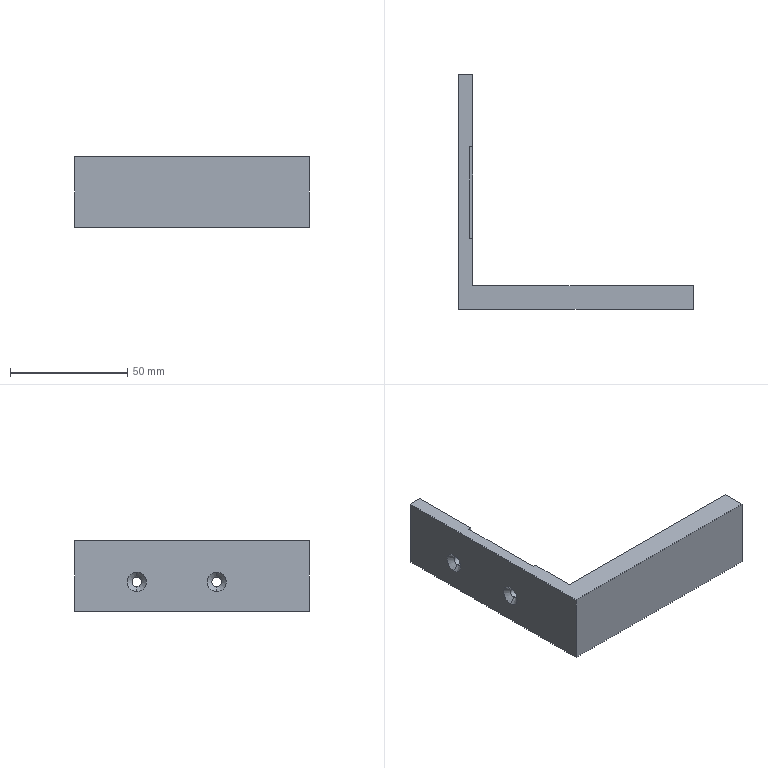Part | SolidWorks | features ICE 2, Chamfer 1, Extrusion 1 | 1 solid | 20 faces | box 100 x 100 x 30 mm | volume 45451 mm3 | plane 12 | cone 4 | cylinder 4 | commonest cylinder face diameters 4 x4
STEP:
#1=CARTESIAN_POINT('',(2.1,73.5,10.5));
#2=VERTEX_POINT('',#1);
#3=CARTESIAN_POINT('',(2.1,73.5,14.5));
#4=VERTEX_POINT('',#3);
#5=CARTESIAN_POINT('',(2.1,73.5,12.5));
#6=DIRECTION('',(-1.,0.,0.));
#7=DIRECTION('',(0.,0.,-1.));
#8=AXIS2_PLACEMENT_3D('',#5,#6,#7);
#9=CIRCLE('',#8,2.);
#10=EDGE_CURVE('',#2,#4,#9,.T.);
#11=ORIENTED_EDGE('',*,*,#10,.F.);
#12=CARTESIAN_POINT('',(0.,73.5,8.4));
#13=VERTEX_POINT('',#12);
#14=CARTESIAN_POINT('',(2.1,73.5,10.5));
#15=DIRECTION('',(-0.7071,0.,-0.7071));
#16=VECTOR('',#15,1000.);
#17=LINE('',#14,#16);
#18=EDGE_CURVE('',#2,#13,#17,.T.);
#19=ORIENTED_EDGE('',*,*,#18,.T.);
#20=CARTESIAN_POINT('',(0.,73.5,16.6));
#21=VERTEX_POINT('',#20);
#22=CARTESIAN_POINT('',(0.,73.5,12.5));
#23=DIRECTION('',(1.,0.,0.));
#24=DIRECTION('',(0.,0.,-1.));
#25=AXIS2_PLACEMENT_3D('',#22,#23,#24);
#26=CIRCLE('',#25,4.1);
#27=EDGE_CURVE('',#21,#13,#26,.T.);
#28=ORIENTED_EDGE('',*,*,#27,.F.);
#29=CARTESIAN_POINT('',(2.1,73.5,14.5));
#30=DIRECTION('',(-0.7071,0.,0.7071));
#31=VECTOR('',#30,1000.);
#32=LINE('',#29,#31);
#33=EDGE_CURVE('',#4,#21,#32,.T.);
#34=ORIENTED_EDGE('',*,*,#33,.F.);
#35=EDGE_LOOP('',(#11,#19,#28,#34));
#36=FACE_OUTER_BOUND('',#35,.T.);
#37=CARTESIAN_POINT('',(2.1,73.5,12.5));
#38=DIRECTION('',(-1.,0.,0.));
#39=DIRECTION('',(0.,0.,1.));
#40=AXIS2_PLACEMENT_3D('',#37,#38,#39);
#41=CONICAL_SURFACE('',#40,2.,0.7854);
#42=ADVANCED_FACE('',(#36),#41,.F.);
#43=CARTESIAN_POINT('',(2.1,39.5,10.5));
#44=VERTEX_POINT('',#43);
#45=CARTESIAN_POINT('',(2.1,39.5,14.5));
#46=VERTEX_POINT('',#45);
#47=CARTESIAN_POINT('',(2.1,39.5,12.5));
#48=DIRECTION('',(-1.,0.,0.));
#49=DIRECTION('',(0.,0.,-1.));
#50=AXIS2_PLACEMENT_3D('',#47,#48,#49);
#51=CIRCLE('',#50,2.);
#52=EDGE_CURVE('',#44,#46,#51,.T.);
#53=ORIENTED_EDGE('',*,*,#52,.F.);
#54=CARTESIAN_POINT('',(0.,39.5,8.4));
#55=VERTEX_POINT('',#54);
#56=CARTESIAN_POINT('',(2.1,39.5,10.5));
#57=DIRECTION('',(-0.7071,0.,-0.7071));
#58=VECTOR('',#57,1000.);
#59=LINE('',#56,#58);
#60=EDGE_CURVE('',#44,#55,#59,.T.);
#61=ORIENTED_EDGE('',*,*,#60,.T.);
#62=CARTESIAN_POINT('',(0.,39.5,16.6));
#63=VERTEX_POINT('',#62);
#64=CARTESIAN_POINT('',(0.,39.5,12.5));
#65=DIRECTION('',(1.,0.,0.));
#66=DIRECTION('',(0.,0.,-1.));
#67=AXIS2_PLACEMENT_3D('',#64,#65,#66);
#68=CIRCLE('',#67,4.1);
#69=EDGE_CURVE('',#63,#55,#68,.T.);
#70=ORIENTED_EDGE('',*,*,#69,.F.);
#71=CARTESIAN_POINT('',(2.1,39.5,14.5));
#72=DIRECTION('',(-0.7071,0.,0.7071));
#73=VECTOR('',#72,1000.);
#74=LINE('',#71,#73);
#75=EDGE_CURVE('',#46,#63,#74,.T.);
#76=ORIENTED_EDGE('',*,*,#75,.F.);
#77=EDGE_LOOP('',(#53,#61,#70,#76));
#78=FACE_OUTER_BOUND('',#77,.T.);
#79=CARTESIAN_POINT('',(2.1,39.5,12.5));
#80=DIRECTION('',(-1.,0.,0.));
#81=DIRECTION('',(0.,0.,1.));
#82=AXIS2_PLACEMENT_3D('',#79,#80,#81);
#83=CONICAL_SURFACE('',#82,2.,0.7854);
#84=ADVANCED_FACE('',(#78),#83,.F.);
#85=CARTESIAN_POINT('',(6.,39.5,10.5));
#86=VERTEX_POINT('',#85);
#87=CARTESIAN_POINT('',(6.,39.5,14.5));
#88=VERTEX_POINT('',#87);
#89=CARTESIAN_POINT('',(6.,39.5,12.5));
#90=DIRECTION('',(-1.,0.,0.));
#91=DIRECTION('',(0.,-1.,0.));
#92=AXIS2_PLACEMENT_3D('',#89,#90,#91);
#93=CIRCLE('',#92,2.);
#94=EDGE_CURVE('',#86,#88,#93,.T.);
#95=ORIENTED_EDGE('',*,*,#94,.F.);
#96=CARTESIAN_POINT('',(100.,39.5,10.5));
#97=DIRECTION('',(-1.,0.,0.));
#98=VECTOR('',#97,1000.);
#99=LINE('',#96,#98);
#100=EDGE_CURVE('',#86,#44,#99,.T.);
#101=ORIENTED_EDGE('',*,*,#100,.T.);
#102=ORIENTED_EDGE('',*,*,#52,.T.);
#103=CARTESIAN_POINT('',(100.,39.5,14.5));
#104=DIRECTION('',(-1.,0.,0.));
#105=VECTOR('',#104,1000.);
#106=LINE('',#103,#105);
#107=EDGE_CURVE('',#88,#46,#106,.T.);
#108=ORIENTED_EDGE('',*,*,#107,.F.);
#109=EDGE_LOOP('',(#95,#101,#102,#108));
#110=FACE_OUTER_BOUND('',#109,.T.);
#111=CARTESIAN_POINT('',(100.,39.5,12.5));
#112=DIRECTION('',(-1.,0.,0.));
#113=DIRECTION('',(0.,0.,1.));
#114=AXIS2_PLACEMENT_3D('',#111,#112,#113);
#115=CYLINDRICAL_SURFACE('',#114,2.);
#116=ADVANCED_FACE('',(#110),#115,.F.);
#117=CARTESIAN_POINT('',(6.,73.5,10.5));
#118=VERTEX_POINT('',#117);
#119=CARTESIAN_POINT('',(6.,73.5,14.5));
#120=VERTEX_POINT('',#119);
#121=CARTESIAN_POINT('',(6.,73.5,12.5));
#122=DIRECTION('',(-1.,0.,0.));
#123=DIRECTION('',(0.,-1.,0.));
#124=AXIS2_PLACEMENT_3D('',#121,#122,#123);
#125=CIRCLE('',#124,2.);
#126=EDGE_CURVE('',#118,#120,#125,.T.);
#127=ORIENTED_EDGE('',*,*,#126,.F.);
#128=CARTESIAN_POINT('',(100.,73.5,10.5));
#129=DIRECTION('',(-1.,0.,0.));
#130=VECTOR('',#129,1000.);
#131=LINE('',#128,#130);
#132=EDGE_CURVE('',#118,#2,#131,.T.);
#133=ORIENTED_EDGE('',*,*,#132,.T.);
#134=ORIENTED_EDGE('',*,*,#10,.T.);
#135=CARTESIAN_POINT('',(100.,73.5,14.5));
#136=DIRECTION('',(-1.,0.,0.));
#137=VECTOR('',#136,1000.);
#138=LINE('',#135,#137);
#139=EDGE_CURVE('',#120,#4,#138,.T.);
#140=ORIENTED_EDGE('',*,*,#139,.F.);
#141=EDGE_LOOP('',(#127,#133,#134,#140));
#142=FACE_OUTER_BOUND('',#141,.T.);
#143=CARTESIAN_POINT('',(100.,73.5,12.5));
#144=DIRECTION('',(-1.,0.,0.));
#145=DIRECTION('',(0.,0.,1.));
#146=AXIS2_PLACEMENT_3D('',#143,#144,#145);
#147=CYLINDRICAL_SURFACE('',#146,2.);
#148=ADVANCED_FACE('',(#142),#147,.F.);
#149=ORIENTED_EDGE('',*,*,#69,.T.);
#150=CARTESIAN_POINT('',(0.,39.5,12.5));
#151=DIRECTION('',(1.,0.,0.));
#152=DIRECTION('',(0.,0.,-1.));
#153=AXIS2_PLACEMENT_3D('',#150,#151,#152);
#154=CIRCLE('',#153,4.1);
#155=EDGE_CURVE('',#55,#63,#154,.T.);
#156=ORIENTED_EDGE('',*,*,#155,.T.);
#157=EDGE_LOOP('',(#149,#156));
#158=FACE_BOUND('',#157,.T.);
#159=ORIENTED_EDGE('',*,*,#27,.T.);
#160=CARTESIAN_POINT('',(0.,73.5,12.5));
#161=DIRECTION('',(1.,0.,0.));
#162=DIRECTION('',(0.,0.,-1.));
#163=AXIS2_PLACEMENT_3D('',#160,#161,#162);
#164=CIRCLE('',#163,4.1);
#165=EDGE_CURVE('',#13,#21,#164,.T.);
#166=ORIENTED_EDGE('',*,*,#165,.T.);
#167=EDGE_LOOP('',(#159,#166));
#168=FACE_BOUND('',#167,.T.);
#169=CARTESIAN_POINT('',(0.,100.,0.));
#170=VERTEX_POINT('',#169);
#171=CARTESIAN_POINT('',(0.,0.,0.));
#172=VERTEX_POINT('',#171);
#173=CARTESIAN_POINT('',(0.,0.,0.));
#174=DIRECTION('',(0.,-1.,0.));
#175=VECTOR('',#174,1000.);
#176=LINE('',#173,#175);
#177=EDGE_CURVE('',#170,#172,#176,.T.);
#178=ORIENTED_EDGE('',*,*,#177,.T.);
#179=CARTESIAN_POINT('',(0.,0.,30.));
#180=VERTEX_POINT('',#179);
#181=CARTESIAN_POINT('',(0.,0.,30.));
#182=DIRECTION('',(0.,0.,-1.));
#183=VECTOR('',#182,1000.);
#184=LINE('',#181,#183);
#185=EDGE_CURVE('',#180,#172,#184,.T.);
#186=ORIENTED_EDGE('',*,*,#185,.F.);
#187=CARTESIAN_POINT('',(0.,100.,30.));
#188=VERTEX_POINT('',#187);
#189=CARTESIAN_POINT('',(0.,0.,30.));
#190=DIRECTION('',(0.,-1.,0.));
#191=VECTOR('',#190,1000.);
#192=LINE('',#189,#191);
#193=EDGE_CURVE('',#188,#180,#192,.T.);
#194=ORIENTED_EDGE('',*,*,#193,.F.);
#195=CARTESIAN_POINT('',(0.,100.,30.));
#196=DIRECTION('',(0.,0.,-1.));
#197=VECTOR('',#196,1000.);
#198=LINE('',#195,#197);
#199=EDGE_CURVE('',#188,#170,#198,.T.);
#200=ORIENTED_EDGE('',*,*,#199,.T.);
#201=EDGE_LOOP('',(#178,#186,#194,#200));
#202=FACE_OUTER_BOUND('',#201,.T.);
#203=CARTESIAN_POINT('',(0.,0.,30.));
#204=DIRECTION('',(1.,0.,0.));
#205=DIRECTION('',(0.,0.,-1.));
#206=AXIS2_PLACEMENT_3D('',#203,#204,#205);
#207=PLANE('',#206);
#208=ADVANCED_FACE('',(#158,#168,#202),#207,.F.);
#209=CARTESIAN_POINT('',(100.,0.,0.));
#210=VERTEX_POINT('',#209);
#211=CARTESIAN_POINT('',(0.,0.,0.));
#212=DIRECTION('',(1.,0.,0.));
#213=VECTOR('',#212,1000.);
#214=LINE('',#211,#213);
#215=EDGE_CURVE('',#172,#210,#214,.T.);
#216=ORIENTED_EDGE('',*,*,#215,.T.);
#217=CARTESIAN_POINT('',(100.,0.,30.));
#218=VERTEX_POINT('',#217);
#219=CARTESIAN_POINT('',(100.,0.,30.));
#220=DIRECTION('',(0.,0.,-1.));
#221=VECTOR('',#220,1000.);
#222=LINE('',#219,#221);
#223=EDGE_CURVE('',#218,#210,#222,.T.);
#224=ORIENTED_EDGE('',*,*,#223,.F.);
#225=CARTESIAN_POINT('',(0.,0.,30.));
#226=DIRECTION('',(1.,0.,0.));
#227=VECTOR('',#226,1000.);
#228=LINE('',#225,#227);
#229=EDGE_CURVE('',#180,#218,#228,.T.);
#230=ORIENTED_EDGE('',*,*,#229,.F.);
#231=ORIENTED_EDGE('',*,*,#185,.T.);
#232=EDGE_LOOP('',(#216,#224,#230,#231));
#233=FACE_OUTER_BOUND('',#232,.T.);
#234=CARTESIAN_POINT('',(0.,0.,30.));
#235=DIRECTION('',(0.,1.,0.));
#236=DIRECTION('',(0.,0.,1.));
#237=AXIS2_PLACEMENT_3D('',#234,#235,#236);
#238=PLANE('',#237);
#239=ADVANCED_FACE('',(#233),#238,.F.);
#240=CARTESIAN_POINT('',(100.,10.,0.));
#241=VERTEX_POINT('',#240);
#242=CARTESIAN_POINT('',(100.,0.,0.));
#243=DIRECTION('',(0.,1.,0.));
#244=VECTOR('',#243,1000.);
#245=LINE('',#242,#244);
#246=EDGE_CURVE('',#210,#241,#245,.T.);
#247=ORIENTED_EDGE('',*,*,#246,.T.);
#248=CARTESIAN_POINT('',(100.,10.,30.));
#249=VERTEX_POINT('',#248);
#250=CARTESIAN_POINT('',(100.,10.,30.));
#251=DIRECTION('',(0.,0.,-1.));
#252=VECTOR('',#251,1000.);
#253=LINE('',#250,#252);
#254=EDGE_CURVE('',#249,#241,#253,.T.);
#255=ORIENTED_EDGE('',*,*,#254,.F.);
#256=CARTESIAN_POINT('',(100.,0.,30.));
#257=DIRECTION('',(0.,1.,0.));
#258=VECTOR('',#257,1000.);
#259=LINE('',#256,#258);
#260=EDGE_CURVE('',#218,#249,#259,.T.);
#261=ORIENTED_EDGE('',*,*,#260,.F.);
#262=ORIENTED_EDGE('',*,*,#223,.T.);
#263=EDGE_LOOP('',(#247,#255,#261,#262));
#264=FACE_OUTER_BOUND('',#263,.T.);
#265=CARTESIAN_POINT('',(100.,0.,30.));
#266=DIRECTION('',(-1.,0.,0.));
#267=DIRECTION('',(0.,0.,1.));
#268=AXIS2_PLACEMENT_3D('',#265,#266,#267);
#269=PLANE('',#268);
#270=ADVANCED_FACE('',(#264),#269,.F.);
#271=CARTESIAN_POINT('',(6.,10.,0.));
#272=VERTEX_POINT('',#271);
#273=CARTESIAN_POINT('',(100.,10.,0.));
#274=DIRECTION('',(-1.,0.,0.));
#275=VECTOR('',#274,1000.);
#276=LINE('',#273,#275);
#277=EDGE_CURVE('',#241,#272,#276,.T.);
#278=ORIENTED_EDGE('',*,*,#277,.T.);
#279=CARTESIAN_POINT('',(6.,10.,30.));
#280=VERTEX_POINT('',#279);
#281=CARTESIAN_POINT('',(6.,10.,30.));
#282=DIRECTION('',(0.,0.,-1.));
#283=VECTOR('',#282,1000.);
#284=LINE('',#281,#283);
#285=EDGE_CURVE('',#280,#272,#284,.T.);
#286=ORIENTED_EDGE('',*,*,#285,.F.);
#287=CARTESIAN_POINT('',(100.,10.,30.));
#288=DIRECTION('',(-1.,0.,0.));
#289=VECTOR('',#288,1000.);
#290=LINE('',#287,#289);
#291=EDGE_CURVE('',#249,#280,#290,.T.);
#292=ORIENTED_EDGE('',*,*,#291,.F.);
#293=ORIENTED_EDGE('',*,*,#254,.T.);
#294=EDGE_LOOP('',(#278,#286,#292,#293));
#295=FACE_OUTER_BOUND('',#294,.T.);
#296=CARTESIAN_POINT('',(100.,10.,30.));
#297=DIRECTION('',(0.,-1.,0.));
#298=DIRECTION('',(1.,0.,0.));
#299=AXIS2_PLACEMENT_3D('',#296,#297,#298);
#300=PLANE('',#299);
#301=ADVANCED_FACE('',(#295),#300,.F.);
#302=CARTESIAN_POINT('',(6.,69.254,30.));
#303=VERTEX_POINT('',#302);
#304=CARTESIAN_POINT('',(6.,100.,30.));
#305=VERTEX_POINT('',#304);
#306=CARTESIAN_POINT('',(6.,10.,30.));
#307=DIRECTION('',(0.,1.,0.));
#308=VECTOR('',#307,1000.);
#309=LINE('',#306,#308);
#310=EDGE_CURVE('',#303,#305,#309,.T.);
#311=ORIENTED_EDGE('',*,*,#310,.F.);
#312=CARTESIAN_POINT('',(6.,69.254,20.));
#313=VERTEX_POINT('',#312);
#314=CARTESIAN_POINT('',(6.,69.254,30.));
#315=DIRECTION('',(0.,0.,-1.));
#316=VECTOR('',#315,1000.);
#317=LINE('',#314,#316);
#318=EDGE_CURVE('',#303,#313,#317,.T.);
#319=ORIENTED_EDGE('',*,*,#318,.T.);
#320=CARTESIAN_POINT('',(6.,30.178,20.));
#321=VERTEX_POINT('',#320);
#322=CARTESIAN_POINT('',(6.,10.,20.));
#323=DIRECTION('',(0.,-1.,0.));
#324=VECTOR('',#323,1000.);
#325=LINE('',#322,#324);
#326=EDGE_CURVE('',#313,#321,#325,.T.);
#327=ORIENTED_EDGE('',*,*,#326,.T.);
#328=CARTESIAN_POINT('',(6.,30.178,30.));
#329=VERTEX_POINT('',#328);
#330=CARTESIAN_POINT('',(6.,30.178,30.));
#331=DIRECTION('',(0.,0.,1.));
#332=VECTOR('',#331,1000.);
#333=LINE('',#330,#332);
#334=EDGE_CURVE('',#321,#329,#333,.T.);
#335=ORIENTED_EDGE('',*,*,#334,.T.);
#336=CARTESIAN_POINT('',(6.,10.,30.));
#337=DIRECTION('',(0.,1.,0.));
#338=VECTOR('',#337,1000.);
#339=LINE('',#336,#338);
#340=EDGE_CURVE('',#280,#329,#339,.T.);
#341=ORIENTED_EDGE('',*,*,#340,.F.);
#342=ORIENTED_EDGE('',*,*,#285,.T.);
#343=CARTESIAN_POINT('',(6.,100.,0.));
#344=VERTEX_POINT('',#343);
#345=CARTESIAN_POINT('',(6.,10.,0.));
#346=DIRECTION('',(0.,1.,0.));
#347=VECTOR('',#346,1000.);
#348=LINE('',#345,#347);
#349=EDGE_CURVE('',#272,#344,#348,.T.);
#350=ORIENTED_EDGE('',*,*,#349,.T.);
#351=CARTESIAN_POINT('',(6.,100.,30.));
#352=DIRECTION('',(0.,0.,-1.));
#353=VECTOR('',#352,1000.);
#354=LINE('',#351,#353);
#355=EDGE_CURVE('',#305,#344,#354,.T.);
#356=ORIENTED_EDGE('',*,*,#355,.F.);
#357=EDGE_LOOP('',(#311,#319,#327,#335,#341,#342,#350,#356));
#358=FACE_OUTER_BOUND('',#357,.T.);
#359=CARTESIAN_POINT('',(6.,39.5,12.5));
#360=DIRECTION('',(-1.,0.,0.));
#361=DIRECTION('',(0.,-1.,0.));
#362=AXIS2_PLACEMENT_3D('',#359,#360,#361);
#363=CIRCLE('',#362,2.);
#364=EDGE_CURVE('',#88,#86,#363,.T.);
#365=ORIENTED_EDGE('',*,*,#364,.T.);
#366=ORIENTED_EDGE('',*,*,#94,.T.);
#367=EDGE_LOOP('',(#365,#366));
#368=FACE_BOUND('',#367,.T.);
#369=CARTESIAN_POINT('',(6.,73.5,12.5));
#370=DIRECTION('',(-1.,0.,0.));
#371=DIRECTION('',(0.,-1.,0.));
#372=AXIS2_PLACEMENT_3D('',#369,#370,#371);
#373=CIRCLE('',#372,2.);
#374=EDGE_CURVE('',#120,#118,#373,.T.);
#375=ORIENTED_EDGE('',*,*,#374,.T.);
#376=ORIENTED_EDGE('',*,*,#126,.T.);
#377=EDGE_LOOP('',(#375,#376));
#378=FACE_BOUND('',#377,.T.);
#379=CARTESIAN_POINT('',(6.,10.,30.));
#380=DIRECTION('',(-1.,0.,0.));
#381=DIRECTION('',(0.,-1.,0.));
#382=AXIS2_PLACEMENT_3D('',#379,#380,#381);
#383=PLANE('',#382);
#384=ADVANCED_FACE('',(#358,#368,#378),#383,.F.);
#385=CARTESIAN_POINT('',(6.,100.,0.));
#386=DIRECTION('',(-1.,0.,0.));
#387=VECTOR('',#386,1000.);
#388=LINE('',#385,#387);
#389=EDGE_CURVE('',#344,#170,#388,.T.);
#390=ORIENTED_EDGE('',*,*,#389,.T.);
#391=ORIENTED_EDGE('',*,*,#199,.F.);
#392=CARTESIAN_POINT('',(6.,100.,30.));
#393=DIRECTION('',(-1.,0.,0.));
#394=VECTOR('',#393,1000.);
#395=LINE('',#392,#394);
#396=EDGE_CURVE('',#305,#188,#395,.T.);
#397=ORIENTED_EDGE('',*,*,#396,.F.);
#398=ORIENTED_EDGE('',*,*,#355,.T.);
#399=EDGE_LOOP('',(#390,#391,#397,#398));
#400=FACE_OUTER_BOUND('',#399,.T.);
#401=CARTESIAN_POINT('',(6.,100.,30.));
#402=DIRECTION('',(0.,-1.,0.));
#403=DIRECTION('',(0.,0.,-1.));
#404=AXIS2_PLACEMENT_3D('',#401,#402,#403);
#405=PLANE('',#404);
#406=ADVANCED_FACE('',(#400),#405,.F.);
#407=CARTESIAN_POINT('',(4.661,69.254,30.));
#408=VERTEX_POINT('',#407);
#409=CARTESIAN_POINT('',(0.,69.254,30.));
#410=DIRECTION('',(-1.,0.,0.));
#411=VECTOR('',#410,1000.);
#412=LINE('',#409,#411);
#413=EDGE_CURVE('',#303,#408,#412,.T.);
#414=ORIENTED_EDGE('',*,*,#413,.F.);
#415=ORIENTED_EDGE('',*,*,#310,.T.);
#416=ORIENTED_EDGE('',*,*,#396,.T.);
#417=ORIENTED_EDGE('',*,*,#193,.T.);
#418=ORIENTED_EDGE('',*,*,#229,.T.);
#419=ORIENTED_EDGE('',*,*,#260,.T.);
#420=ORIENTED_EDGE('',*,*,#291,.T.);
#421=ORIENTED_EDGE('',*,*,#340,.T.);
#422=CARTESIAN_POINT('',(4.661,30.178,30.));
#423=VERTEX_POINT('',#422);
#424=CARTESIAN_POINT('',(7.339,30.178,30.));
#425=DIRECTION('',(1.,0.,0.));
#426=VECTOR('',#425,1000.);
#427=LINE('',#424,#426);
#428=EDGE_CURVE('',#423,#329,#427,.T.);
#429=ORIENTED_EDGE('',*,*,#428,.F.);
#430=CARTESIAN_POINT('',(4.661,69.254,30.));
#431=DIRECTION('',(0.,-1.,0.));
#432=VECTOR('',#431,1000.);
#433=LINE('',#430,#432);
#434=EDGE_CURVE('',#408,#423,#433,.T.);
#435=ORIENTED_EDGE('',*,*,#434,.F.);
#436=EDGE_LOOP('',(#414,#415,#416,#417,#418,#419,#420,#421,#429,#435));
#437=FACE_OUTER_BOUND('',#436,.T.);
#438=CARTESIAN_POINT('',(0.,0.,30.));
#439=DIRECTION('',(0.,0.,1.));
#440=DIRECTION('',(1.,0.,0.));
#441=AXIS2_PLACEMENT_3D('',#438,#439,#440);
#442=PLANE('',#441);
#443=ADVANCED_FACE('',(#437),#442,.T.);
#444=ORIENTED_EDGE('',*,*,#177,.F.);
#445=ORIENTED_EDGE('',*,*,#389,.F.);
#446=ORIENTED_EDGE('',*,*,#349,.F.);
#447=ORIENTED_EDGE('',*,*,#277,.F.);
#448=ORIENTED_EDGE('',*,*,#246,.F.);
#449=ORIENTED_EDGE('',*,*,#215,.F.);
#450=EDGE_LOOP('',(#444,#445,#446,#447,#448,#449));
#451=FACE_OUTER_BOUND('',#450,.T.);
#452=CARTESIAN_POINT('',(0.,0.,0.));
#453=DIRECTION('',(0.,0.,1.));
#454=DIRECTION('',(1.,0.,0.));
#455=AXIS2_PLACEMENT_3D('',#452,#453,#454);
#456=PLANE('',#455);
#457=ADVANCED_FACE('',(#451),#456,.F.);
#458=ORIENTED_EDGE('',*,*,#132,.F.);
#459=ORIENTED_EDGE('',*,*,#374,.F.);
#460=ORIENTED_EDGE('',*,*,#139,.T.);
#461=CARTESIAN_POINT('',(2.1,73.5,12.5));
#462=DIRECTION('',(-1.,0.,0.));
#463=DIRECTION('',(0.,0.,-1.));
#464=AXIS2_PLACEMENT_3D('',#461,#462,#463);
#465=CIRCLE('',#464,2.);
#466=EDGE_CURVE('',#4,#2,#465,.T.);
#467=ORIENTED_EDGE('',*,*,#466,.T.);
#468=EDGE_LOOP('',(#458,#459,#460,#467));
#469=FACE_OUTER_BOUND('',#468,.T.);
#470=CARTESIAN_POINT('',(100.,73.5,12.5));
#471=DIRECTION('',(-1.,0.,0.));
#472=DIRECTION('',(0.,0.,1.));
#473=AXIS2_PLACEMENT_3D('',#470,#471,#472);
#474=CYLINDRICAL_SURFACE('',#473,2.);
#475=ADVANCED_FACE('',(#469),#474,.F.);
#476=ORIENTED_EDGE('',*,*,#100,.F.);
#477=ORIENTED_EDGE('',*,*,#364,.F.);
#478=ORIENTED_EDGE('',*,*,#107,.T.);
#479=CARTESIAN_POINT('',(2.1,39.5,12.5));
#480=DIRECTION('',(-1.,0.,0.));
#481=DIRECTION('',(0.,0.,-1.));
#482=AXIS2_PLACEMENT_3D('',#479,#480,#481);
#483=CIRCLE('',#482,2.);
#484=EDGE_CURVE('',#46,#44,#483,.T.);
#485=ORIENTED_EDGE('',*,*,#484,.T.);
#486=EDGE_LOOP('',(#476,#477,#478,#485));
#487=FACE_OUTER_BOUND('',#486,.T.);
#488=CARTESIAN_POINT('',(100.,39.5,12.5));
#489=DIRECTION('',(-1.,0.,0.));
#490=DIRECTION('',(0.,0.,1.));
#491=AXIS2_PLACEMENT_3D('',#488,#489,#490);
#492=CYLINDRICAL_SURFACE('',#491,2.);
#493=ADVANCED_FACE('',(#487),#492,.F.);
#494=ORIENTED_EDGE('',*,*,#60,.F.);
#495=ORIENTED_EDGE('',*,*,#484,.F.);
#496=ORIENTED_EDGE('',*,*,#75,.T.);
#497=ORIENTED_EDGE('',*,*,#155,.F.);
#498=EDGE_LOOP('',(#494,#495,#496,#497));
#499=FACE_OUTER_BOUND('',#498,.T.);
#500=CARTESIAN_POINT('',(2.1,39.5,12.5));
#501=DIRECTION('',(-1.,0.,0.));
#502=DIRECTION('',(0.,0.,1.));
#503=AXIS2_PLACEMENT_3D('',#500,#501,#502);
#504=CONICAL_SURFACE('',#503,2.,0.7854);
#505=ADVANCED_FACE('',(#499),#504,.F.);
#506=ORIENTED_EDGE('',*,*,#18,.F.);
#507=ORIENTED_EDGE('',*,*,#466,.F.);
#508=ORIENTED_EDGE('',*,*,#33,.T.);
#509=ORIENTED_EDGE('',*,*,#165,.F.);
#510=EDGE_LOOP('',(#506,#507,#508,#509));
#511=FACE_OUTER_BOUND('',#510,.T.);
#512=CARTESIAN_POINT('',(2.1,73.5,12.5));
#513=DIRECTION('',(-1.,0.,0.));
#514=DIRECTION('',(0.,0.,1.));
#515=AXIS2_PLACEMENT_3D('',#512,#513,#514);
#516=CONICAL_SURFACE('',#515,2.,0.7854);
#517=ADVANCED_FACE('',(#511),#516,.F.);
#518=CARTESIAN_POINT('',(4.661,69.254,20.));
#519=VERTEX_POINT('',#518);
#520=CARTESIAN_POINT('',(7.339,69.254,20.));
#521=DIRECTION('',(-1.,0.,0.));
#522=VECTOR('',#521,1000.);
#523=LINE('',#520,#522);
#524=EDGE_CURVE('',#313,#519,#523,.T.);
#525=ORIENTED_EDGE('',*,*,#524,.T.);
#526=CARTESIAN_POINT('',(4.661,30.178,20.));
#527=VERTEX_POINT('',#526);
#528=CARTESIAN_POINT('',(4.661,69.254,20.));
#529=DIRECTION('',(0.,-1.,0.));
#530=VECTOR('',#529,1000.);
#531=LINE('',#528,#530);
#532=EDGE_CURVE('',#519,#527,#531,.T.);
#533=ORIENTED_EDGE('',*,*,#532,.T.);
#534=CARTESIAN_POINT('',(7.339,30.178,20.));
#535=DIRECTION('',(1.,0.,0.));
#536=VECTOR('',#535,1000.);
#537=LINE('',#534,#536);
#538=EDGE_CURVE('',#527,#321,#537,.T.);
#539=ORIENTED_EDGE('',*,*,#538,.T.);
#540=ORIENTED_EDGE('',*,*,#326,.F.);
#541=EDGE_LOOP('',(#525,#533,#539,#540));
#542=FACE_OUTER_BOUND('',#541,.T.);
#543=CARTESIAN_POINT('',(0.,0.,20.));
#544=DIRECTION('',(0.,0.,-1.));
#545=DIRECTION('',(-1.,0.,0.));
#546=AXIS2_PLACEMENT_3D('',#543,#544,#545);
#547=PLANE('',#546);
#548=ADVANCED_FACE('',(#542),#547,.F.);
#549=ORIENTED_EDGE('',*,*,#413,.T.);
#550=CARTESIAN_POINT('',(4.661,69.254,20.));
#551=DIRECTION('',(0.,0.,1.));
#552=VECTOR('',#551,1000.);
#553=LINE('',#550,#552);
#554=EDGE_CURVE('',#519,#408,#553,.T.);
#555=ORIENTED_EDGE('',*,*,#554,.F.);
#556=ORIENTED_EDGE('',*,*,#524,.F.);
#557=ORIENTED_EDGE('',*,*,#318,.F.);
#558=EDGE_LOOP('',(#549,#555,#556,#557));
#559=FACE_OUTER_BOUND('',#558,.T.);
#560=CARTESIAN_POINT('',(7.339,69.254,20.));
#561=DIRECTION('',(0.,1.,0.));
#562=DIRECTION('',(0.,0.,1.));
#563=AXIS2_PLACEMENT_3D('',#560,#561,#562);
#564=PLANE('',#563);
#565=ADVANCED_FACE('',(#559),#564,.F.);
#566=ORIENTED_EDGE('',*,*,#538,.F.);
#567=CARTESIAN_POINT('',(4.661,30.178,20.));
#568=DIRECTION('',(0.,0.,1.));
#569=VECTOR('',#568,1000.);
#570=LINE('',#567,#569);
#571=EDGE_CURVE('',#527,#423,#570,.T.);
#572=ORIENTED_EDGE('',*,*,#571,.T.);
#573=ORIENTED_EDGE('',*,*,#428,.T.);
#574=ORIENTED_EDGE('',*,*,#334,.F.);
#575=EDGE_LOOP('',(#566,#572,#573,#574));
#576=FACE_OUTER_BOUND('',#575,.T.);
#577=CARTESIAN_POINT('',(7.339,30.178,20.));
#578=DIRECTION('',(0.,-1.,0.));
#579=DIRECTION('',(0.,0.,-1.));
#580=AXIS2_PLACEMENT_3D('',#577,#578,#579);
#581=PLANE('',#580);
#582=ADVANCED_FACE('',(#576),#581,.F.);
#583=ORIENTED_EDGE('',*,*,#434,.T.);
#584=ORIENTED_EDGE('',*,*,#571,.F.);
#585=ORIENTED_EDGE('',*,*,#532,.F.);
#586=ORIENTED_EDGE('',*,*,#554,.T.);
#587=EDGE_LOOP('',(#583,#584,#585,#586));
#588=FACE_OUTER_BOUND('',#587,.T.);
#589=CARTESIAN_POINT('',(4.661,69.254,20.));
#590=DIRECTION('',(-1.,0.,0.));
#591=DIRECTION('',(0.,-1.,0.));
#592=AXIS2_PLACEMENT_3D('',#589,#590,#591);
#593=PLANE('',#592);
#594=ADVANCED_FACE('',(#588),#593,.F.);
#595=CLOSED_SHELL('',(#42,#84,#116,#148,#208,#239,#270,#301,#384,#406,#443,#457,#475,#493,#505,#517,#548,#565,#582,#594));
#596=MANIFOLD_SOLID_BREP('',#595);
#597=CARTESIAN_POINT('',(0.,0.,0.));
#598=DIRECTION('',(0.,0.,1.));
#599=DIRECTION('',(1.,0.,0.));
#600=AXIS2_PLACEMENT_3D('',#597,#598,#599);
#601=(LENGTH_UNIT()NAMED_UNIT(*)SI_UNIT(.MILLI.,.METRE.));
#602=UNCERTAINTY_MEASURE_WITH_UNIT(LENGTH_MEASURE(0.00001),#601,'','');
#603=(NAMED_UNIT(*)PLANE_ANGLE_UNIT()SI_UNIT($,.RADIAN.));
#604=(NAMED_UNIT(*)SI_UNIT($,.STERADIAN.)SOLID_ANGLE_UNIT());
#605=(GEOMETRIC_REPRESENTATION_CONTEXT(3)GLOBAL_UNCERTAINTY_ASSIGNED_CONTEXT((#602))GLOBAL_UNIT_ASSIGNED_CONTEXT((#601,#603,#604))REPRESENTATION_CONTEXT('',''));
#606=ADVANCED_BREP_SHAPE_REPRESENTATION('',(#596,#600),#605);